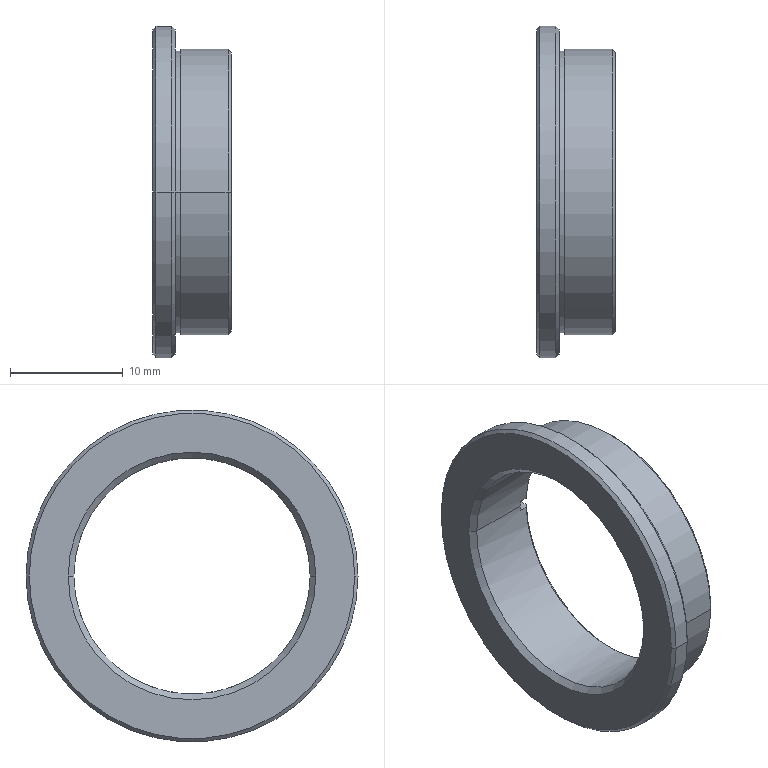Part | STEP file | pressure ring 4.stp.STEP-242.STEP | 1 solid | 30 faces | box 7 x 29.5 x 29.5 mm | volume 1442 mm3 | cylinder 10 | cone 10 | plane 10 | commonest cylinder face diameters 1 x2 21 x2 25 x2 25.4 x2 29.5 x2
STEP:
#1=CARTESIAN_POINT('',(435.04,-10.5,0.));
#2=VERTEX_POINT('',#1);
#3=CARTESIAN_POINT('',(435.04,10.5,0.));
#4=VERTEX_POINT('',#3);
#5=CARTESIAN_POINT('',(435.04,0.,0.));
#6=DIRECTION('',(-1.,0.,0.));
#7=DIRECTION('',(0.,-1.,0.));
#8=AXIS2_PLACEMENT_3D('',#5,#6,#7);
#9=CIRCLE('',#8,10.5);
#10=EDGE_CURVE('',#2,#4,#9,.T.);
#11=ORIENTED_EDGE('',*,*,#10,.T.);
#12=CARTESIAN_POINT('',(440.54,10.5,0.));
#13=VERTEX_POINT('',#12);
#14=CARTESIAN_POINT('',(0.,10.5,0.));
#15=DIRECTION('',(1.,0.,0.));
#16=VECTOR('',#15,1000.);
#17=LINE('',#14,#16);
#18=EDGE_CURVE('',#4,#13,#17,.T.);
#19=ORIENTED_EDGE('',*,*,#18,.T.);
#20=CARTESIAN_POINT('',(440.54,10.488,0.5));
#21=VERTEX_POINT('',#20);
#22=CARTESIAN_POINT('',(440.54,0.,0.));
#23=DIRECTION('',(-1.,0.,0.));
#24=DIRECTION('',(0.,0.,1.));
#25=AXIS2_PLACEMENT_3D('',#22,#23,#24);
#26=CIRCLE('',#25,10.5);
#27=EDGE_CURVE('',#21,#13,#26,.T.);
#28=ORIENTED_EDGE('',*,*,#27,.F.);
#29=CARTESIAN_POINT('',(441.24,10.488,0.5));
#30=VERTEX_POINT('',#29);
#31=CARTESIAN_POINT('',(0.,10.488,0.5));
#32=DIRECTION('',(1.,0.,0.));
#33=VECTOR('',#32,1000.);
#34=LINE('',#31,#33);
#35=EDGE_CURVE('',#21,#30,#34,.T.);
#36=ORIENTED_EDGE('',*,*,#35,.T.);
#37=CARTESIAN_POINT('',(441.24,-10.488,0.5));
#38=VERTEX_POINT('',#37);
#39=CARTESIAN_POINT('',(441.24,0.,0.));
#40=DIRECTION('',(1.,0.,0.));
#41=DIRECTION('',(0.,1.,0.));
#42=AXIS2_PLACEMENT_3D('',#39,#40,#41);
#43=CIRCLE('',#42,10.5);
#44=EDGE_CURVE('',#30,#38,#43,.T.);
#45=ORIENTED_EDGE('',*,*,#44,.T.);
#46=CARTESIAN_POINT('',(440.54,-10.488,0.5));
#47=VERTEX_POINT('',#46);
#48=CARTESIAN_POINT('',(0.,-10.488,0.5));
#49=DIRECTION('',(-1.,0.,0.));
#50=VECTOR('',#49,1000.);
#51=LINE('',#48,#50);
#52=EDGE_CURVE('',#38,#47,#51,.T.);
#53=ORIENTED_EDGE('',*,*,#52,.T.);
#54=CARTESIAN_POINT('',(440.54,-10.5,0.));
#55=VERTEX_POINT('',#54);
#56=CARTESIAN_POINT('',(440.54,0.,0.));
#57=DIRECTION('',(-1.,0.,0.));
#58=DIRECTION('',(0.,0.,1.));
#59=AXIS2_PLACEMENT_3D('',#56,#57,#58);
#60=CIRCLE('',#59,10.5);
#61=EDGE_CURVE('',#55,#47,#60,.T.);
#62=ORIENTED_EDGE('',*,*,#61,.F.);
#63=CARTESIAN_POINT('',(0.,-10.5,0.));
#64=DIRECTION('',(1.,0.,0.));
#65=VECTOR('',#64,1000.);
#66=LINE('',#63,#65);
#67=EDGE_CURVE('',#2,#55,#66,.T.);
#68=ORIENTED_EDGE('',*,*,#67,.F.);
#69=EDGE_LOOP('',(#11,#19,#28,#36,#45,#53,#62,#68));
#70=FACE_OUTER_BOUND('',#69,.T.);
#71=CARTESIAN_POINT('',(0.,0.,0.));
#72=DIRECTION('',(1.,0.,0.));
#73=DIRECTION('',(0.,-1.,0.));
#74=AXIS2_PLACEMENT_3D('',#71,#72,#73);
#75=CYLINDRICAL_SURFACE('',#74,10.5);
#76=ADVANCED_FACE('',(#70),#75,.F.);
#77=CARTESIAN_POINT('',(436.54,-12.5,0.));
#78=VERTEX_POINT('',#77);
#79=CARTESIAN_POINT('',(436.54,12.5,0.));
#80=VERTEX_POINT('',#79);
#81=CARTESIAN_POINT('',(436.54,0.,0.));
#82=DIRECTION('',(1.,0.,0.));
#83=DIRECTION('',(0.,-1.,0.));
#84=AXIS2_PLACEMENT_3D('',#81,#82,#83);
#85=CIRCLE('',#84,12.5);
#86=EDGE_CURVE('',#78,#80,#85,.T.);
#87=ORIENTED_EDGE('',*,*,#86,.T.);
#88=CARTESIAN_POINT('',(437.04,12.5,0.));
#89=VERTEX_POINT('',#88);
#90=CARTESIAN_POINT('',(0.,12.5,0.));
#91=DIRECTION('',(1.,0.,0.));
#92=VECTOR('',#91,1000.);
#93=LINE('',#90,#92);
#94=EDGE_CURVE('',#80,#89,#93,.T.);
#95=ORIENTED_EDGE('',*,*,#94,.T.);
#96=CARTESIAN_POINT('',(437.04,-12.5,0.));
#97=VERTEX_POINT('',#96);
#98=CARTESIAN_POINT('',(437.04,0.,0.));
#99=DIRECTION('',(1.,0.,0.));
#100=DIRECTION('',(0.,-1.,0.));
#101=AXIS2_PLACEMENT_3D('',#98,#99,#100);
#102=CIRCLE('',#101,12.5);
#103=EDGE_CURVE('',#97,#89,#102,.T.);
#104=ORIENTED_EDGE('',*,*,#103,.F.);
#105=CARTESIAN_POINT('',(0.,-12.5,0.));
#106=DIRECTION('',(1.,0.,0.));
#107=VECTOR('',#106,1000.);
#108=LINE('',#105,#107);
#109=EDGE_CURVE('',#78,#97,#108,.T.);
#110=ORIENTED_EDGE('',*,*,#109,.F.);
#111=EDGE_LOOP('',(#87,#95,#104,#110));
#112=FACE_OUTER_BOUND('',#111,.T.);
#113=CARTESIAN_POINT('',(0.,0.,0.));
#114=DIRECTION('',(1.,0.,0.));
#115=DIRECTION('',(0.,-1.,0.));
#116=AXIS2_PLACEMENT_3D('',#113,#114,#115);
#117=CYLINDRICAL_SURFACE('',#116,12.5);
#118=ADVANCED_FACE('',(#112),#117,.T.);
#119=CARTESIAN_POINT('',(434.84,-14.75,0.));
#120=VERTEX_POINT('',#119);
#121=CARTESIAN_POINT('',(434.84,14.75,0.));
#122=VERTEX_POINT('',#121);
#123=CARTESIAN_POINT('',(434.84,0.,0.));
#124=DIRECTION('',(1.,0.,0.));
#125=DIRECTION('',(0.,-1.,0.));
#126=AXIS2_PLACEMENT_3D('',#123,#124,#125);
#127=CIRCLE('',#126,14.75);
#128=EDGE_CURVE('',#120,#122,#127,.T.);
#129=ORIENTED_EDGE('',*,*,#128,.T.);
#130=CARTESIAN_POINT('',(436.24,14.75,0.));
#131=VERTEX_POINT('',#130);
#132=CARTESIAN_POINT('',(0.,14.75,0.));
#133=DIRECTION('',(1.,0.,0.));
#134=VECTOR('',#133,1000.);
#135=LINE('',#132,#134);
#136=EDGE_CURVE('',#122,#131,#135,.T.);
#137=ORIENTED_EDGE('',*,*,#136,.T.);
#138=CARTESIAN_POINT('',(436.24,-14.75,0.));
#139=VERTEX_POINT('',#138);
#140=CARTESIAN_POINT('',(436.24,0.,0.));
#141=DIRECTION('',(-1.,0.,0.));
#142=DIRECTION('',(0.,1.,0.));
#143=AXIS2_PLACEMENT_3D('',#140,#141,#142);
#144=CIRCLE('',#143,14.75);
#145=EDGE_CURVE('',#131,#139,#144,.T.);
#146=ORIENTED_EDGE('',*,*,#145,.T.);
#147=CARTESIAN_POINT('',(0.,-14.75,0.));
#148=DIRECTION('',(1.,0.,0.));
#149=VECTOR('',#148,1000.);
#150=LINE('',#147,#149);
#151=EDGE_CURVE('',#120,#139,#150,.T.);
#152=ORIENTED_EDGE('',*,*,#151,.F.);
#153=EDGE_LOOP('',(#129,#137,#146,#152));
#154=FACE_OUTER_BOUND('',#153,.T.);
#155=CARTESIAN_POINT('',(0.,0.,0.));
#156=DIRECTION('',(1.,0.,0.));
#157=DIRECTION('',(0.,-1.,0.));
#158=AXIS2_PLACEMENT_3D('',#155,#156,#157);
#159=CYLINDRICAL_SURFACE('',#158,14.75);
#160=ADVANCED_FACE('',(#154),#159,.T.);
#161=CARTESIAN_POINT('',(437.04,-12.7,0.));
#162=VERTEX_POINT('',#161);
#163=CARTESIAN_POINT('',(437.04,12.7,0.));
#164=VERTEX_POINT('',#163);
#165=CARTESIAN_POINT('',(437.04,0.,0.));
#166=DIRECTION('',(1.,0.,0.));
#167=DIRECTION('',(0.,-1.,0.));
#168=AXIS2_PLACEMENT_3D('',#165,#166,#167);
#169=CIRCLE('',#168,12.7);
#170=EDGE_CURVE('',#162,#164,#169,.T.);
#171=ORIENTED_EDGE('',*,*,#170,.T.);
#172=CARTESIAN_POINT('',(441.24,12.7,0.));
#173=VERTEX_POINT('',#172);
#174=CARTESIAN_POINT('',(0.,12.7,0.));
#175=DIRECTION('',(1.,0.,0.));
#176=VECTOR('',#175,1000.);
#177=LINE('',#174,#176);
#178=EDGE_CURVE('',#164,#173,#177,.T.);
#179=ORIENTED_EDGE('',*,*,#178,.T.);
#180=CARTESIAN_POINT('',(441.24,-12.7,0.));
#181=VERTEX_POINT('',#180);
#182=CARTESIAN_POINT('',(441.24,0.,0.));
#183=DIRECTION('',(-1.,0.,0.));
#184=DIRECTION('',(0.,1.,0.));
#185=AXIS2_PLACEMENT_3D('',#182,#183,#184);
#186=CIRCLE('',#185,12.7);
#187=EDGE_CURVE('',#173,#181,#186,.T.);
#188=ORIENTED_EDGE('',*,*,#187,.T.);
#189=CARTESIAN_POINT('',(0.,-12.7,0.));
#190=DIRECTION('',(1.,0.,0.));
#191=VECTOR('',#190,1000.);
#192=LINE('',#189,#191);
#193=EDGE_CURVE('',#162,#181,#192,.T.);
#194=ORIENTED_EDGE('',*,*,#193,.F.);
#195=EDGE_LOOP('',(#171,#179,#188,#194));
#196=FACE_OUTER_BOUND('',#195,.T.);
#197=CARTESIAN_POINT('',(0.,0.,0.));
#198=DIRECTION('',(1.,0.,0.));
#199=DIRECTION('',(0.,-1.,0.));
#200=AXIS2_PLACEMENT_3D('',#197,#198,#199);
#201=CYLINDRICAL_SURFACE('',#200,12.7);
#202=ADVANCED_FACE('',(#196),#201,.T.);
#203=CARTESIAN_POINT('',(436.54,14.45,0.));
#204=VERTEX_POINT('',#203);
#205=CARTESIAN_POINT('',(436.54,-14.45,0.));
#206=VERTEX_POINT('',#205);
#207=CARTESIAN_POINT('',(436.54,0.,0.));
#208=DIRECTION('',(1.,0.,0.));
#209=DIRECTION('',(0.,1.,0.));
#210=AXIS2_PLACEMENT_3D('',#207,#208,#209);
#211=CIRCLE('',#210,14.45);
#212=EDGE_CURVE('',#204,#206,#211,.T.);
#213=ORIENTED_EDGE('',*,*,#212,.F.);
#214=CARTESIAN_POINT('',(436.54,14.45,0.));
#215=DIRECTION('',(-0.7071,0.7071,0.));
#216=VECTOR('',#215,1000.);
#217=LINE('',#214,#216);
#218=EDGE_CURVE('',#204,#131,#217,.T.);
#219=ORIENTED_EDGE('',*,*,#218,.T.);
#220=CARTESIAN_POINT('',(436.24,0.,0.));
#221=DIRECTION('',(-1.,0.,0.));
#222=DIRECTION('',(0.,1.,0.));
#223=AXIS2_PLACEMENT_3D('',#220,#221,#222);
#224=CIRCLE('',#223,14.75);
#225=EDGE_CURVE('',#139,#131,#224,.T.);
#226=ORIENTED_EDGE('',*,*,#225,.F.);
#227=CARTESIAN_POINT('',(436.54,-14.45,0.));
#228=DIRECTION('',(-0.7071,-0.7071,0.));
#229=VECTOR('',#228,1000.);
#230=LINE('',#227,#229);
#231=EDGE_CURVE('',#206,#139,#230,.T.);
#232=ORIENTED_EDGE('',*,*,#231,.F.);
#233=EDGE_LOOP('',(#213,#219,#226,#232));
#234=FACE_OUTER_BOUND('',#233,.T.);
#235=CARTESIAN_POINT('',(436.54,0.,0.));
#236=DIRECTION('',(-1.,0.,0.));
#237=DIRECTION('',(0.,-1.,0.));
#238=AXIS2_PLACEMENT_3D('',#235,#236,#237);
#239=CONICAL_SURFACE('',#238,14.45,0.7854);
#240=ADVANCED_FACE('',(#234),#239,.T.);
#241=CARTESIAN_POINT('',(434.54,-14.45,0.));
#242=VERTEX_POINT('',#241);
#243=CARTESIAN_POINT('',(434.54,14.45,0.));
#244=VERTEX_POINT('',#243);
#245=CARTESIAN_POINT('',(434.54,0.,0.));
#246=DIRECTION('',(-1.,0.,0.));
#247=DIRECTION('',(0.,-1.,0.));
#248=AXIS2_PLACEMENT_3D('',#245,#246,#247);
#249=CIRCLE('',#248,14.45);
#250=EDGE_CURVE('',#242,#244,#249,.T.);
#251=ORIENTED_EDGE('',*,*,#250,.F.);
#252=CARTESIAN_POINT('',(434.84,-14.75,0.));
#253=DIRECTION('',(0.7071,-0.7071,0.));
#254=VECTOR('',#253,1000.);
#255=LINE('',#252,#254);
#256=EDGE_CURVE('',#242,#120,#255,.T.);
#257=ORIENTED_EDGE('',*,*,#256,.T.);
#258=CARTESIAN_POINT('',(434.84,0.,0.));
#259=DIRECTION('',(1.,0.,0.));
#260=DIRECTION('',(0.,-1.,0.));
#261=AXIS2_PLACEMENT_3D('',#258,#259,#260);
#262=CIRCLE('',#261,14.75);
#263=EDGE_CURVE('',#122,#120,#262,.T.);
#264=ORIENTED_EDGE('',*,*,#263,.F.);
#265=CARTESIAN_POINT('',(434.84,14.75,0.));
#266=DIRECTION('',(0.7071,0.7071,0.));
#267=VECTOR('',#266,1000.);
#268=LINE('',#265,#267);
#269=EDGE_CURVE('',#244,#122,#268,.T.);
#270=ORIENTED_EDGE('',*,*,#269,.F.);
#271=EDGE_LOOP('',(#251,#257,#264,#270));
#272=FACE_OUTER_BOUND('',#271,.T.);
#273=CARTESIAN_POINT('',(434.84,0.,0.));
#274=DIRECTION('',(1.,0.,0.));
#275=DIRECTION('',(0.,1.,0.));
#276=AXIS2_PLACEMENT_3D('',#273,#274,#275);
#277=CONICAL_SURFACE('',#276,14.75,0.7854);
#278=ADVANCED_FACE('',(#272),#277,.T.);
#279=CARTESIAN_POINT('',(441.54,12.4,0.));
#280=VERTEX_POINT('',#279);
#281=CARTESIAN_POINT('',(441.54,-12.4,0.));
#282=VERTEX_POINT('',#281);
#283=CARTESIAN_POINT('',(441.54,0.,0.));
#284=DIRECTION('',(1.,0.,0.));
#285=DIRECTION('',(0.,1.,0.));
#286=AXIS2_PLACEMENT_3D('',#283,#284,#285);
#287=CIRCLE('',#286,12.4);
#288=EDGE_CURVE('',#280,#282,#287,.T.);
#289=ORIENTED_EDGE('',*,*,#288,.F.);
#290=CARTESIAN_POINT('',(441.54,12.4,0.));
#291=DIRECTION('',(-0.7071,0.7071,0.));
#292=VECTOR('',#291,1000.);
#293=LINE('',#290,#292);
#294=EDGE_CURVE('',#280,#173,#293,.T.);
#295=ORIENTED_EDGE('',*,*,#294,.T.);
#296=CARTESIAN_POINT('',(441.24,0.,0.));
#297=DIRECTION('',(-1.,0.,0.));
#298=DIRECTION('',(0.,1.,0.));
#299=AXIS2_PLACEMENT_3D('',#296,#297,#298);
#300=CIRCLE('',#299,12.7);
#301=EDGE_CURVE('',#181,#173,#300,.T.);
#302=ORIENTED_EDGE('',*,*,#301,.F.);
#303=CARTESIAN_POINT('',(441.54,-12.4,0.));
#304=DIRECTION('',(-0.7071,-0.7071,0.));
#305=VECTOR('',#304,1000.);
#306=LINE('',#303,#305);
#307=EDGE_CURVE('',#282,#181,#306,.T.);
#308=ORIENTED_EDGE('',*,*,#307,.F.);
#309=EDGE_LOOP('',(#289,#295,#302,#308));
#310=FACE_OUTER_BOUND('',#309,.T.);
#311=CARTESIAN_POINT('',(441.54,0.,0.));
#312=DIRECTION('',(-1.,0.,0.));
#313=DIRECTION('',(0.,-1.,0.));
#314=AXIS2_PLACEMENT_3D('',#311,#312,#313);
#315=CONICAL_SURFACE('',#314,12.4,0.7854);
#316=ADVANCED_FACE('',(#310),#315,.T.);
#317=CARTESIAN_POINT('',(435.04,0.,0.));
#318=DIRECTION('',(-1.,0.,0.));
#319=DIRECTION('',(0.,-1.,0.));
#320=AXIS2_PLACEMENT_3D('',#317,#318,#319);
#321=CIRCLE('',#320,10.5);
#322=EDGE_CURVE('',#4,#2,#321,.T.);
#323=ORIENTED_EDGE('',*,*,#322,.F.);
#324=CARTESIAN_POINT('',(434.54,11.,0.));
#325=VERTEX_POINT('',#324);
#326=CARTESIAN_POINT('',(434.54,11.,0.));
#327=DIRECTION('',(-0.7071,0.7071,0.));
#328=VECTOR('',#327,1000.);
#329=LINE('',#326,#328);
#330=EDGE_CURVE('',#4,#325,#329,.T.);
#331=ORIENTED_EDGE('',*,*,#330,.T.);
#332=CARTESIAN_POINT('',(434.54,-11.,0.));
#333=VERTEX_POINT('',#332);
#334=CARTESIAN_POINT('',(434.54,0.,0.));
#335=DIRECTION('',(1.,0.,0.));
#336=DIRECTION('',(0.,-1.,0.));
#337=AXIS2_PLACEMENT_3D('',#334,#335,#336);
#338=CIRCLE('',#337,11.);
#339=EDGE_CURVE('',#333,#325,#338,.T.);
#340=ORIENTED_EDGE('',*,*,#339,.F.);
#341=CARTESIAN_POINT('',(434.54,-11.,0.));
#342=DIRECTION('',(-0.7071,-0.7071,0.));
#343=VECTOR('',#342,1000.);
#344=LINE('',#341,#343);
#345=EDGE_CURVE('',#2,#333,#344,.T.);
#346=ORIENTED_EDGE('',*,*,#345,.F.);
#347=EDGE_LOOP('',(#323,#331,#340,#346));
#348=FACE_OUTER_BOUND('',#347,.T.);
#349=CARTESIAN_POINT('',(434.54,0.,0.));
#350=DIRECTION('',(-1.,0.,0.));
#351=DIRECTION('',(0.,-1.,0.));
#352=AXIS2_PLACEMENT_3D('',#349,#350,#351);
#353=CONICAL_SURFACE('',#352,11.,0.7854);
#354=ADVANCED_FACE('',(#348),#353,.F.);
#355=CARTESIAN_POINT('',(440.54,-10.488,-0.5));
#356=VERTEX_POINT('',#355);
#357=CARTESIAN_POINT('',(440.54,0.,0.));
#358=DIRECTION('',(-1.,0.,0.));
#359=DIRECTION('',(0.,0.,1.));
#360=AXIS2_PLACEMENT_3D('',#357,#358,#359);
#361=CIRCLE('',#360,10.5);
#362=EDGE_CURVE('',#356,#55,#361,.T.);
#363=ORIENTED_EDGE('',*,*,#362,.T.);
#364=ORIENTED_EDGE('',*,*,#61,.T.);
#365=CARTESIAN_POINT('',(440.54,-11.5,0.5));
#366=VERTEX_POINT('',#365);
#367=CARTESIAN_POINT('',(440.54,11.5,0.5));
#368=DIRECTION('',(0.,-1.,0.));
#369=VECTOR('',#368,1000.);
#370=LINE('',#367,#369);
#371=EDGE_CURVE('',#47,#366,#370,.T.);
#372=ORIENTED_EDGE('',*,*,#371,.T.);
#373=CARTESIAN_POINT('',(440.54,-11.5,-0.5));
#374=VERTEX_POINT('',#373);
#375=CARTESIAN_POINT('',(440.54,-11.5,0.));
#376=DIRECTION('',(1.,0.,0.));
#377=DIRECTION('',(0.,0.,-1.));
#378=AXIS2_PLACEMENT_3D('',#375,#376,#377);
#379=CIRCLE('',#378,0.5);
#380=EDGE_CURVE('',#366,#374,#379,.T.);
#381=ORIENTED_EDGE('',*,*,#380,.T.);
#382=CARTESIAN_POINT('',(440.54,-11.5,-0.5));
#383=DIRECTION('',(0.,1.,0.));
#384=VECTOR('',#383,1000.);
#385=LINE('',#382,#384);
#386=EDGE_CURVE('',#374,#356,#385,.T.);
#387=ORIENTED_EDGE('',*,*,#386,.T.);
#388=EDGE_LOOP('',(#363,#364,#372,#381,#387));
#389=FACE_OUTER_BOUND('',#388,.T.);
#390=CARTESIAN_POINT('',(440.54,-11.5,0.));
#391=DIRECTION('',(-1.,0.,0.));
#392=DIRECTION('',(0.,0.,1.));
#393=AXIS2_PLACEMENT_3D('',#390,#391,#392);
#394=PLANE('',#393);
#395=ADVANCED_FACE('',(#389),#394,.F.);
#396=ORIENTED_EDGE('',*,*,#330,.F.);
#397=ORIENTED_EDGE('',*,*,#10,.F.);
#398=ORIENTED_EDGE('',*,*,#345,.T.);
#399=CARTESIAN_POINT('',(434.54,0.,0.));
#400=DIRECTION('',(1.,0.,0.));
#401=DIRECTION('',(0.,-1.,0.));
#402=AXIS2_PLACEMENT_3D('',#399,#400,#401);
#403=CIRCLE('',#402,11.);
#404=EDGE_CURVE('',#325,#333,#403,.T.);
#405=ORIENTED_EDGE('',*,*,#404,.F.);
#406=EDGE_LOOP('',(#396,#397,#398,#405));
#407=FACE_OUTER_BOUND('',#406,.T.);
#408=CARTESIAN_POINT('',(434.54,0.,0.));
#409=DIRECTION('',(-1.,0.,0.));
#410=DIRECTION('',(0.,-1.,0.));
#411=AXIS2_PLACEMENT_3D('',#408,#409,#410);
#412=CONICAL_SURFACE('',#411,11.,0.7854);
#413=ADVANCED_FACE('',(#407),#412,.F.);
#414=CARTESIAN_POINT('',(441.54,10.788,0.5));
#415=VERTEX_POINT('',#414);
#416=CARTESIAN_POINT('',(441.54,10.788,0.5));
#417=CARTESIAN_POINT('',(441.44,10.688,0.5));
#418=CARTESIAN_POINT('',(441.34,10.588,0.5));
#419=CARTESIAN_POINT('',(441.24,10.488,0.5));
#420=B_SPLINE_CURVE_WITH_KNOTS('',3,(#416,#417,#418,#419),.UNSPECIFIED.,.F.,.F.,(4,4),(0.,0.0004245),.UNSPECIFIED.);
#421=EDGE_CURVE('',#415,#30,#420,.T.);
#422=ORIENTED_EDGE('',*,*,#421,.F.);
#423=CARTESIAN_POINT('',(441.54,-10.788,0.5));
#424=VERTEX_POINT('',#423);
#425=CARTESIAN_POINT('',(441.54,0.,0.));
#426=DIRECTION('',(-1.,0.,0.));
#427=DIRECTION('',(0.,1.,0.));
#428=AXIS2_PLACEMENT_3D('',#425,#426,#427);
#429=CIRCLE('',#428,10.8);
#430=EDGE_CURVE('',#424,#415,#429,.T.);
#431=ORIENTED_EDGE('',*,*,#430,.F.);
#432=CARTESIAN_POINT('',(441.24,-10.488,0.5));
#433=CARTESIAN_POINT('',(441.34,-10.588,0.5));
#434=CARTESIAN_POINT('',(441.44,-10.688,0.5));
#435=CARTESIAN_POINT('',(441.54,-10.788,0.5));
#436=B_SPLINE_CURVE_WITH_KNOTS('',3,(#432,#433,#434,#435),.UNSPECIFIED.,.F.,.F.,(4,4),(0.,0.0004245),.UNSPECIFIED.);
#437=EDGE_CURVE('',#38,#424,#436,.T.);
#438=ORIENTED_EDGE('',*,*,#437,.F.);
#439=ORIENTED_EDGE('',*,*,#44,.F.);
#440=EDGE_LOOP('',(#422,#431,#438,#439));
#441=FACE_OUTER_BOUND('',#440,.T.);
#442=CARTESIAN_POINT('',(441.24,0.,0.));
#443=DIRECTION('',(1.,0.,0.));
#444=DIRECTION('',(0.,1.,0.));
#445=AXIS2_PLACEMENT_3D('',#442,#443,#444);
#446=CONICAL_SURFACE('',#445,10.5,0.7854);
#447=ADVANCED_FACE('',(#441),#446,.F.);
#448=ORIENTED_EDGE('',*,*,#294,.F.);
#449=CARTESIAN_POINT('',(441.54,0.,0.));
#450=DIRECTION('',(1.,0.,0.));
#451=DIRECTION('',(0.,1.,0.));
#452=AXIS2_PLACEMENT_3D('',#449,#450,#451);
#453=CIRCLE('',#452,12.4);
#454=EDGE_CURVE('',#282,#280,#453,.T.);
#455=ORIENTED_EDGE('',*,*,#454,.F.);
#456=ORIENTED_EDGE('',*,*,#307,.T.);
#457=ORIENTED_EDGE('',*,*,#187,.F.);
#458=EDGE_LOOP('',(#448,#455,#456,#457));
#459=FACE_OUTER_BOUND('',#458,.T.);
#460=CARTESIAN_POINT('',(441.54,0.,0.));
#461=DIRECTION('',(-1.,0.,0.));
#462=DIRECTION('',(0.,-1.,0.));
#463=AXIS2_PLACEMENT_3D('',#460,#461,#462);
#464=CONICAL_SURFACE('',#463,12.4,0.7854);
#465=ADVANCED_FACE('',(#459),#464,.T.);
#466=ORIENTED_EDGE('',*,*,#256,.F.);
#467=CARTESIAN_POINT('',(434.54,0.,0.));
#468=DIRECTION('',(-1.,0.,0.));
#469=DIRECTION('',(0.,-1.,0.));
#470=AXIS2_PLACEMENT_3D('',#467,#468,#469);
#471=CIRCLE('',#470,14.45);
#472=EDGE_CURVE('',#244,#242,#471,.T.);
#473=ORIENTED_EDGE('',*,*,#472,.F.);
#474=ORIENTED_EDGE('',*,*,#269,.T.);
#475=ORIENTED_EDGE('',*,*,#128,.F.);
#476=EDGE_LOOP('',(#466,#473,#474,#475));
#477=FACE_OUTER_BOUND('',#476,.T.);
#478=CARTESIAN_POINT('',(434.84,0.,0.));
#479=DIRECTION('',(1.,0.,0.));
#480=DIRECTION('',(0.,1.,0.));
#481=AXIS2_PLACEMENT_3D('',#478,#479,#480);
#482=CONICAL_SURFACE('',#481,14.75,0.7854);
#483=ADVANCED_FACE('',(#477),#482,.T.);
#484=ORIENTED_EDGE('',*,*,#218,.F.);
#485=CARTESIAN_POINT('',(436.54,0.,0.));
#486=DIRECTION('',(1.,0.,0.));
#487=DIRECTION('',(0.,1.,0.));
#488=AXIS2_PLACEMENT_3D('',#485,#486,#487);
#489=CIRCLE('',#488,14.45);
#490=EDGE_CURVE('',#206,#204,#489,.T.);
#491=ORIENTED_EDGE('',*,*,#490,.F.);
#492=ORIENTED_EDGE('',*,*,#231,.T.);
#493=ORIENTED_EDGE('',*,*,#145,.F.);
#494=EDGE_LOOP('',(#484,#491,#492,#493));
#495=FACE_OUTER_BOUND('',#494,.T.);
#496=CARTESIAN_POINT('',(436.54,0.,0.));
#497=DIRECTION('',(-1.,0.,0.));
#498=DIRECTION('',(0.,-1.,0.));
#499=AXIS2_PLACEMENT_3D('',#496,#497,#498);
#500=CONICAL_SURFACE('',#499,14.45,0.7854);
#501=ADVANCED_FACE('',(#495),#500,.T.);
#502=CARTESIAN_POINT('',(441.54,11.5,0.5));
#503=VERTEX_POINT('',#502);
#504=CARTESIAN_POINT('',(441.54,11.5,0.5));
#505=DIRECTION('',(0.,-1.,0.));
#506=VECTOR('',#505,1000.);
#507=LINE('',#504,#506);
#508=EDGE_CURVE('',#503,#415,#507,.T.);
#509=ORIENTED_EDGE('',*,*,#508,.T.);
#510=ORIENTED_EDGE('',*,*,#421,.T.);
#511=ORIENTED_EDGE('',*,*,#35,.F.);
#512=CARTESIAN_POINT('',(440.54,11.5,0.5));
#513=VERTEX_POINT('',#512);
#514=CARTESIAN_POINT('',(440.54,11.5,0.5));
#515=DIRECTION('',(0.,-1.,0.));
#516=VECTOR('',#515,1000.);
#517=LINE('',#514,#516);
#518=EDGE_CURVE('',#513,#21,#517,.T.);
#519=ORIENTED_EDGE('',*,*,#518,.F.);
#520=CARTESIAN_POINT('',(440.54,11.5,0.5));
#521=DIRECTION('',(1.,0.,0.));
#522=VECTOR('',#521,1000.);
#523=LINE('',#520,#522);
#524=EDGE_CURVE('',#513,#503,#523,.T.);
#525=ORIENTED_EDGE('',*,*,#524,.T.);
#526=EDGE_LOOP('',(#509,#510,#511,#519,#525));
#527=FACE_OUTER_BOUND('',#526,.T.);
#528=CARTESIAN_POINT('',(440.54,11.5,0.5));
#529=DIRECTION('',(0.,0.,-1.));
#530=DIRECTION('',(0.,-1.,0.));
#531=AXIS2_PLACEMENT_3D('',#528,#529,#530);
#532=PLANE('',#531);
#533=ADVANCED_FACE('',(#527),#532,.T.);
#534=CARTESIAN_POINT('',(441.24,10.488,-0.5));
#535=VERTEX_POINT('',#534);
#536=CARTESIAN_POINT('',(440.54,10.488,-0.5));
#537=VERTEX_POINT('',#536);
#538=CARTESIAN_POINT('',(0.,10.488,-0.5));
#539=DIRECTION('',(-1.,0.,0.));
#540=VECTOR('',#539,1000.);
#541=LINE('',#538,#540);
#542=EDGE_CURVE('',#535,#537,#541,.T.);
#543=ORIENTED_EDGE('',*,*,#542,.F.);
#544=CARTESIAN_POINT('',(441.54,10.788,-0.5));
#545=VERTEX_POINT('',#544);
#546=CARTESIAN_POINT('',(441.24,10.488,-0.5));
#547=CARTESIAN_POINT('',(441.34,10.588,-0.5));
#548=CARTESIAN_POINT('',(441.44,10.688,-0.5));
#549=CARTESIAN_POINT('',(441.54,10.788,-0.5));
#550=B_SPLINE_CURVE_WITH_KNOTS('',3,(#546,#547,#548,#549),.UNSPECIFIED.,.F.,.F.,(4,4),(0.,0.0004245),.UNSPECIFIED.);
#551=EDGE_CURVE('',#535,#545,#550,.T.);
#552=ORIENTED_EDGE('',*,*,#551,.T.);
#553=CARTESIAN_POINT('',(441.54,11.5,-0.5));
#554=VERTEX_POINT('',#553);
#555=CARTESIAN_POINT('',(441.54,-11.5,-0.5));
#556=DIRECTION('',(0.,1.,0.));
#557=VECTOR('',#556,1000.);
#558=LINE('',#555,#557);
#559=EDGE_CURVE('',#545,#554,#558,.T.);
#560=ORIENTED_EDGE('',*,*,#559,.T.);
#561=CARTESIAN_POINT('',(440.54,11.5,-0.5));
#562=VERTEX_POINT('',#561);
#563=CARTESIAN_POINT('',(440.54,11.5,-0.5));
#564=DIRECTION('',(1.,0.,0.));
#565=VECTOR('',#564,1000.);
#566=LINE('',#563,#565);
#567=EDGE_CURVE('',#562,#554,#566,.T.);
#568=ORIENTED_EDGE('',*,*,#567,.F.);
#569=CARTESIAN_POINT('',(440.54,-11.5,-0.5));
#570=DIRECTION('',(0.,1.,0.));
#571=VECTOR('',#570,1000.);
#572=LINE('',#569,#571);
#573=EDGE_CURVE('',#537,#562,#572,.T.);
#574=ORIENTED_EDGE('',*,*,#573,.F.);
#575=EDGE_LOOP('',(#543,#552,#560,#568,#574));
#576=FACE_OUTER_BOUND('',#575,.T.);
#577=CARTESIAN_POINT('',(440.54,-11.5,-0.5));
#578=DIRECTION('',(0.,0.,1.));
#579=DIRECTION('',(1.,0.,0.));
#580=AXIS2_PLACEMENT_3D('',#577,#578,#579);
#581=PLANE('',#580);
#582=ADVANCED_FACE('',(#576),#581,.T.);
#583=CARTESIAN_POINT('',(441.54,-11.5,-0.5));
#584=VERTEX_POINT('',#583);
#585=CARTESIAN_POINT('',(441.54,-10.788,-0.5));
#586=VERTEX_POINT('',#585);
#587=CARTESIAN_POINT('',(441.54,-11.5,-0.5));
#588=DIRECTION('',(0.,1.,0.));
#589=VECTOR('',#588,1000.);
#590=LINE('',#587,#589);
#591=EDGE_CURVE('',#584,#586,#590,.T.);
#592=ORIENTED_EDGE('',*,*,#591,.T.);
#593=CARTESIAN_POINT('',(441.24,-10.488,-0.5));
#594=VERTEX_POINT('',#593);
#595=CARTESIAN_POINT('',(441.54,-10.788,-0.5));
#596=CARTESIAN_POINT('',(441.44,-10.688,-0.5));
#597=CARTESIAN_POINT('',(441.34,-10.588,-0.5));
#598=CARTESIAN_POINT('',(441.24,-10.488,-0.5));
#599=B_SPLINE_CURVE_WITH_KNOTS('',3,(#595,#596,#597,#598),.UNSPECIFIED.,.F.,.F.,(4,4),(0.,0.0004245),.UNSPECIFIED.);
#600=EDGE_CURVE('',#586,#594,#599,.T.);
#601=ORIENTED_EDGE('',*,*,#600,.T.);
#602=CARTESIAN_POINT('',(0.,-10.488,-0.5));
#603=DIRECTION('',(1.,0.,0.));
#604=VECTOR('',#603,1000.);
#605=LINE('',#602,#604);
#606=EDGE_CURVE('',#356,#594,#605,.T.);
#607=ORIENTED_EDGE('',*,*,#606,.F.);
#608=ORIENTED_EDGE('',*,*,#386,.F.);
#609=CARTESIAN_POINT('',(440.54,-11.5,-0.5));
#610=DIRECTION('',(1.,0.,0.));
#611=VECTOR('',#610,1000.);
#612=LINE('',#609,#611);
#613=EDGE_CURVE('',#374,#584,#612,.T.);
#614=ORIENTED_EDGE('',*,*,#613,.T.);
#615=EDGE_LOOP('',(#592,#601,#607,#608,#614));
#616=FACE_OUTER_BOUND('',#615,.T.);
#617=CARTESIAN_POINT('',(440.54,-11.5,-0.5));
#618=DIRECTION('',(0.,0.,1.));
#619=DIRECTION('',(1.,0.,0.));
#620=AXIS2_PLACEMENT_3D('',#617,#618,#619);
#621=PLANE('',#620);
#622=ADVANCED_FACE('',(#616),#621,.T.);
#623=CARTESIAN_POINT('',(441.54,-11.5,0.5));
#624=VERTEX_POINT('',#623);
#625=CARTESIAN_POINT('',(441.54,-11.5,0.));
#626=DIRECTION('',(1.,0.,0.));
#627=DIRECTION('',(0.,0.,-1.));
#628=AXIS2_PLACEMENT_3D('',#625,#626,#627);
#629=CIRCLE('',#628,0.5);
#630=EDGE_CURVE('',#624,#584,#629,.T.);
#631=ORIENTED_EDGE('',*,*,#630,.T.);
#632=ORIENTED_EDGE('',*,*,#613,.F.);
#633=ORIENTED_EDGE('',*,*,#380,.F.);
#634=CARTESIAN_POINT('',(440.54,-11.5,0.5));
#635=DIRECTION('',(1.,0.,0.));
#636=VECTOR('',#635,1000.);
#637=LINE('',#634,#636);
#638=EDGE_CURVE('',#366,#624,#637,.T.);
#639=ORIENTED_EDGE('',*,*,#638,.T.);
#640=EDGE_LOOP('',(#631,#632,#633,#639));
#641=FACE_OUTER_BOUND('',#640,.T.);
#642=CARTESIAN_POINT('',(440.54,-11.5,0.));
#643=DIRECTION('',(1.,0.,0.));
#644=DIRECTION('',(0.,0.,1.));
#645=AXIS2_PLACEMENT_3D('',#642,#643,#644);
#646=CYLINDRICAL_SURFACE('',#645,0.5);
#647=ADVANCED_FACE('',(#641),#646,.F.);
#648=ORIENTED_EDGE('',*,*,#559,.F.);
#649=CARTESIAN_POINT('',(441.54,0.,0.));
#650=DIRECTION('',(-1.,0.,0.));
#651=DIRECTION('',(0.,1.,0.));
#652=AXIS2_PLACEMENT_3D('',#649,#650,#651);
#653=CIRCLE('',#652,10.8);
#654=EDGE_CURVE('',#545,#586,#653,.T.);
#655=ORIENTED_EDGE('',*,*,#654,.T.);
#656=ORIENTED_EDGE('',*,*,#591,.F.);
#657=ORIENTED_EDGE('',*,*,#630,.F.);
#658=CARTESIAN_POINT('',(441.54,11.5,0.5));
#659=DIRECTION('',(0.,-1.,0.));
#660=VECTOR('',#659,1000.);
#661=LINE('',#658,#660);
#662=EDGE_CURVE('',#424,#624,#661,.T.);
#663=ORIENTED_EDGE('',*,*,#662,.F.);
#664=ORIENTED_EDGE('',*,*,#430,.T.);
#665=ORIENTED_EDGE('',*,*,#508,.F.);
#666=CARTESIAN_POINT('',(441.54,11.5,0.));
#667=DIRECTION('',(1.,0.,0.));
#668=DIRECTION('',(0.,0.,-1.));
#669=AXIS2_PLACEMENT_3D('',#666,#667,#668);
#670=CIRCLE('',#669,0.5);
#671=EDGE_CURVE('',#554,#503,#670,.T.);
#672=ORIENTED_EDGE('',*,*,#671,.F.);
#673=EDGE_LOOP('',(#648,#655,#656,#657,#663,#664,#665,#672));
#674=FACE_BOUND('',#673,.T.);
#675=ORIENTED_EDGE('',*,*,#454,.T.);
#676=ORIENTED_EDGE('',*,*,#288,.T.);
#677=EDGE_LOOP('',(#675,#676));
#678=FACE_OUTER_BOUND('',#677,.T.);
#679=CARTESIAN_POINT('',(441.54,10.5,0.));
#680=DIRECTION('',(1.,0.,0.));
#681=DIRECTION('',(0.,1.,0.));
#682=AXIS2_PLACEMENT_3D('',#679,#680,#681);
#683=PLANE('',#682);
#684=ADVANCED_FACE('',(#674,#678),#683,.T.);
#685=ORIENTED_EDGE('',*,*,#178,.F.);
#686=CARTESIAN_POINT('',(437.04,0.,0.));
#687=DIRECTION('',(1.,0.,0.));
#688=DIRECTION('',(0.,-1.,0.));
#689=AXIS2_PLACEMENT_3D('',#686,#687,#688);
#690=CIRCLE('',#689,12.7);
#691=EDGE_CURVE('',#164,#162,#690,.T.);
#692=ORIENTED_EDGE('',*,*,#691,.T.);
#693=ORIENTED_EDGE('',*,*,#193,.T.);
#694=ORIENTED_EDGE('',*,*,#301,.T.);
#695=EDGE_LOOP('',(#685,#692,#693,#694));
#696=FACE_OUTER_BOUND('',#695,.T.);
#697=CARTESIAN_POINT('',(0.,0.,0.));
#698=DIRECTION('',(1.,0.,0.));
#699=DIRECTION('',(0.,-1.,0.));
#700=AXIS2_PLACEMENT_3D('',#697,#698,#699);
#701=CYLINDRICAL_SURFACE('',#700,12.7);
#702=ADVANCED_FACE('',(#696),#701,.T.);
#703=ORIENTED_EDGE('',*,*,#86,.F.);
#704=CARTESIAN_POINT('',(436.54,0.,0.));
#705=DIRECTION('',(1.,0.,0.));
#706=DIRECTION('',(0.,-1.,0.));
#707=AXIS2_PLACEMENT_3D('',#704,#705,#706);
#708=CIRCLE('',#707,12.5);
#709=EDGE_CURVE('',#80,#78,#708,.T.);
#710=ORIENTED_EDGE('',*,*,#709,.F.);
#711=EDGE_LOOP('',(#703,#710));
#712=FACE_BOUND('',#711,.T.);
#713=ORIENTED_EDGE('',*,*,#490,.T.);
#714=ORIENTED_EDGE('',*,*,#212,.T.);
#715=EDGE_LOOP('',(#713,#714));
#716=FACE_OUTER_BOUND('',#715,.T.);
#717=CARTESIAN_POINT('',(436.54,12.5,0.));
#718=DIRECTION('',(1.,0.,0.));
#719=DIRECTION('',(0.,1.,0.));
#720=AXIS2_PLACEMENT_3D('',#717,#718,#719);
#721=PLANE('',#720);
#722=ADVANCED_FACE('',(#712,#716),#721,.T.);
#723=ORIENTED_EDGE('',*,*,#136,.F.);
#724=ORIENTED_EDGE('',*,*,#263,.T.);
#725=ORIENTED_EDGE('',*,*,#151,.T.);
#726=ORIENTED_EDGE('',*,*,#225,.T.);
#727=EDGE_LOOP('',(#723,#724,#725,#726));
#728=FACE_OUTER_BOUND('',#727,.T.);
#729=CARTESIAN_POINT('',(0.,0.,0.));
#730=DIRECTION('',(1.,0.,0.));
#731=DIRECTION('',(0.,-1.,0.));
#732=AXIS2_PLACEMENT_3D('',#729,#730,#731);
#733=CYLINDRICAL_SURFACE('',#732,14.75);
#734=ADVANCED_FACE('',(#728),#733,.T.);
#735=ORIENTED_EDGE('',*,*,#339,.T.);
#736=ORIENTED_EDGE('',*,*,#404,.T.);
#737=EDGE_LOOP('',(#735,#736));
#738=FACE_BOUND('',#737,.T.);
#739=ORIENTED_EDGE('',*,*,#472,.T.);
#740=ORIENTED_EDGE('',*,*,#250,.T.);
#741=EDGE_LOOP('',(#739,#740));
#742=FACE_OUTER_BOUND('',#741,.T.);
#743=CARTESIAN_POINT('',(434.54,14.75,0.));
#744=DIRECTION('',(-1.,0.,0.));
#745=DIRECTION('',(0.,1.,0.));
#746=AXIS2_PLACEMENT_3D('',#743,#744,#745);
#747=PLANE('',#746);
#748=ADVANCED_FACE('',(#738,#742),#747,.T.);
#749=ORIENTED_EDGE('',*,*,#94,.F.);
#750=ORIENTED_EDGE('',*,*,#709,.T.);
#751=ORIENTED_EDGE('',*,*,#109,.T.);
#752=CARTESIAN_POINT('',(437.04,0.,0.));
#753=DIRECTION('',(1.,0.,0.));
#754=DIRECTION('',(0.,-1.,0.));
#755=AXIS2_PLACEMENT_3D('',#752,#753,#754);
#756=CIRCLE('',#755,12.5);
#757=EDGE_CURVE('',#89,#97,#756,.T.);
#758=ORIENTED_EDGE('',*,*,#757,.F.);
#759=EDGE_LOOP('',(#749,#750,#751,#758));
#760=FACE_OUTER_BOUND('',#759,.T.);
#761=CARTESIAN_POINT('',(0.,0.,0.));
#762=DIRECTION('',(1.,0.,0.));
#763=DIRECTION('',(0.,-1.,0.));
#764=AXIS2_PLACEMENT_3D('',#761,#762,#763);
#765=CYLINDRICAL_SURFACE('',#764,12.5);
#766=ADVANCED_FACE('',(#760),#765,.T.);
#767=ORIENTED_EDGE('',*,*,#18,.F.);
#768=ORIENTED_EDGE('',*,*,#322,.T.);
#769=ORIENTED_EDGE('',*,*,#67,.T.);
#770=ORIENTED_EDGE('',*,*,#362,.F.);
#771=ORIENTED_EDGE('',*,*,#606,.T.);
#772=CARTESIAN_POINT('',(441.24,0.,0.));
#773=DIRECTION('',(1.,0.,0.));
#774=DIRECTION('',(0.,1.,0.));
#775=AXIS2_PLACEMENT_3D('',#772,#773,#774);
#776=CIRCLE('',#775,10.5);
#777=EDGE_CURVE('',#594,#535,#776,.T.);
#778=ORIENTED_EDGE('',*,*,#777,.T.);
#779=ORIENTED_EDGE('',*,*,#542,.T.);
#780=CARTESIAN_POINT('',(440.54,0.,0.));
#781=DIRECTION('',(-1.,0.,0.));
#782=DIRECTION('',(0.,0.,1.));
#783=AXIS2_PLACEMENT_3D('',#780,#781,#782);
#784=CIRCLE('',#783,10.5);
#785=EDGE_CURVE('',#13,#537,#784,.T.);
#786=ORIENTED_EDGE('',*,*,#785,.F.);
#787=EDGE_LOOP('',(#767,#768,#769,#770,#771,#778,#779,#786));
#788=FACE_OUTER_BOUND('',#787,.T.);
#789=CARTESIAN_POINT('',(0.,0.,0.));
#790=DIRECTION('',(1.,0.,0.));
#791=DIRECTION('',(0.,-1.,0.));
#792=AXIS2_PLACEMENT_3D('',#789,#790,#791);
#793=CYLINDRICAL_SURFACE('',#792,10.5);
#794=ADVANCED_FACE('',(#788),#793,.F.);
#795=ORIENTED_EDGE('',*,*,#103,.T.);
#796=ORIENTED_EDGE('',*,*,#757,.T.);
#797=EDGE_LOOP('',(#795,#796));
#798=FACE_BOUND('',#797,.T.);
#799=ORIENTED_EDGE('',*,*,#170,.F.);
#800=ORIENTED_EDGE('',*,*,#691,.F.);
#801=EDGE_LOOP('',(#799,#800));
#802=FACE_OUTER_BOUND('',#801,.T.);
#803=CARTESIAN_POINT('',(437.04,12.7,0.));
#804=DIRECTION('',(-1.,0.,0.));
#805=DIRECTION('',(0.,1.,0.));
#806=AXIS2_PLACEMENT_3D('',#803,#804,#805);
#807=PLANE('',#806);
#808=ADVANCED_FACE('',(#798,#802),#807,.T.);
#809=ORIENTED_EDGE('',*,*,#27,.T.);
#810=ORIENTED_EDGE('',*,*,#785,.T.);
#811=ORIENTED_EDGE('',*,*,#573,.T.);
#812=CARTESIAN_POINT('',(440.54,11.5,0.));
#813=DIRECTION('',(1.,0.,0.));
#814=DIRECTION('',(0.,0.,-1.));
#815=AXIS2_PLACEMENT_3D('',#812,#813,#814);
#816=CIRCLE('',#815,0.5);
#817=EDGE_CURVE('',#562,#513,#816,.T.);
#818=ORIENTED_EDGE('',*,*,#817,.T.);
#819=ORIENTED_EDGE('',*,*,#518,.T.);
#820=EDGE_LOOP('',(#809,#810,#811,#818,#819));
#821=FACE_OUTER_BOUND('',#820,.T.);
#822=CARTESIAN_POINT('',(440.54,-11.5,0.));
#823=DIRECTION('',(-1.,0.,0.));
#824=DIRECTION('',(0.,0.,1.));
#825=AXIS2_PLACEMENT_3D('',#822,#823,#824);
#826=PLANE('',#825);
#827=ADVANCED_FACE('',(#821),#826,.F.);
#828=ORIENTED_EDGE('',*,*,#671,.T.);
#829=ORIENTED_EDGE('',*,*,#524,.F.);
#830=ORIENTED_EDGE('',*,*,#817,.F.);
#831=ORIENTED_EDGE('',*,*,#567,.T.);
#832=EDGE_LOOP('',(#828,#829,#830,#831));
#833=FACE_OUTER_BOUND('',#832,.T.);
#834=CARTESIAN_POINT('',(440.54,11.5,0.));
#835=DIRECTION('',(1.,0.,0.));
#836=DIRECTION('',(0.,0.,1.));
#837=AXIS2_PLACEMENT_3D('',#834,#835,#836);
#838=CYLINDRICAL_SURFACE('',#837,0.5);
#839=ADVANCED_FACE('',(#833),#838,.F.);
#840=ORIENTED_EDGE('',*,*,#52,.F.);
#841=ORIENTED_EDGE('',*,*,#437,.T.);
#842=ORIENTED_EDGE('',*,*,#662,.T.);
#843=ORIENTED_EDGE('',*,*,#638,.F.);
#844=ORIENTED_EDGE('',*,*,#371,.F.);
#845=EDGE_LOOP('',(#840,#841,#842,#843,#844));
#846=FACE_OUTER_BOUND('',#845,.T.);
#847=CARTESIAN_POINT('',(440.54,11.5,0.5));
#848=DIRECTION('',(0.,0.,-1.));
#849=DIRECTION('',(0.,-1.,0.));
#850=AXIS2_PLACEMENT_3D('',#847,#848,#849);
#851=PLANE('',#850);
#852=ADVANCED_FACE('',(#846),#851,.T.);
#853=ORIENTED_EDGE('',*,*,#600,.F.);
#854=ORIENTED_EDGE('',*,*,#654,.F.);
#855=ORIENTED_EDGE('',*,*,#551,.F.);
#856=ORIENTED_EDGE('',*,*,#777,.F.);
#857=EDGE_LOOP('',(#853,#854,#855,#856));
#858=FACE_OUTER_BOUND('',#857,.T.);
#859=CARTESIAN_POINT('',(441.24,0.,0.));
#860=DIRECTION('',(1.,0.,0.));
#861=DIRECTION('',(0.,1.,0.));
#862=AXIS2_PLACEMENT_3D('',#859,#860,#861);
#863=CONICAL_SURFACE('',#862,10.5,0.7854);
#864=ADVANCED_FACE('',(#858),#863,.F.);
#865=CLOSED_SHELL('',(#76,#118,#160,#202,#240,#278,#316,#354,#395,#413,#447,#465,#483,#501,#533,#582,#622,#647,#684,#702,#722,#734,#748,#766,#794,#808,#827,#839,#852,#864));
#866=MANIFOLD_SOLID_BREP('',#865);
#867=CARTESIAN_POINT('',(0.,0.,0.));
#868=DIRECTION('',(0.,0.,1.));
#869=DIRECTION('',(1.,0.,0.));
#870=AXIS2_PLACEMENT_3D('',#867,#868,#869);
#871=(LENGTH_UNIT()NAMED_UNIT(*)SI_UNIT(.MILLI.,.METRE.));
#872=UNCERTAINTY_MEASURE_WITH_UNIT(LENGTH_MEASURE(0.00001),#871,'','');
#873=(NAMED_UNIT(*)PLANE_ANGLE_UNIT()SI_UNIT($,.RADIAN.));
#874=(NAMED_UNIT(*)SI_UNIT($,.STERADIAN.)SOLID_ANGLE_UNIT());
#875=(GEOMETRIC_REPRESENTATION_CONTEXT(3)GLOBAL_UNCERTAINTY_ASSIGNED_CONTEXT((#872))GLOBAL_UNIT_ASSIGNED_CONTEXT((#871,#873,#874))REPRESENTATION_CONTEXT('',''));
#876=ADVANCED_BREP_SHAPE_REPRESENTATION('',(#866,#870),#875);